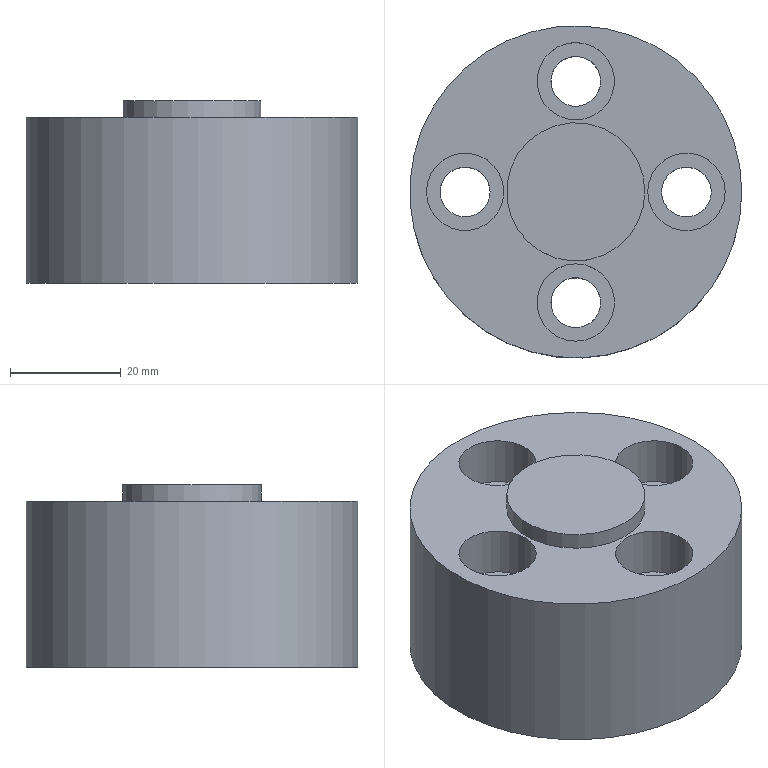Part | NX | 1 solid | 17 faces | box 60 x 60 x 33 mm | volume 75410 mm3 | cylinder 10 | plane 7 | commonest cylinder face diameters 9 x4 14 x4 25 x1 60 x1
STEP:
#1=CARTESIAN_POINT('',(0.,-24.5,-30.));
#2=VERTEX_POINT('',#1);
#3=CARTESIAN_POINT('',(0.,-20.,-30.));
#4=DIRECTION('',(0.,0.,1.));
#5=DIRECTION('',(0.,-1.,0.));
#6=AXIS2_PLACEMENT_3D('',#3,#4,#5);
#7=CIRCLE('',#6,4.5);
#8=EDGE_CURVE('',#2,#2,#7,.T.);
#9=ORIENTED_EDGE('',*,*,#8,.F.);
#10=EDGE_LOOP('',(#9));
#11=FACE_BOUND('',#10,.T.);
#12=CARTESIAN_POINT('',(4.5,-20.,-9.));
#13=VERTEX_POINT('',#12);
#14=CARTESIAN_POINT('',(0.,-20.,-9.));
#15=DIRECTION('',(0.,0.,1.));
#16=DIRECTION('',(1.,0.,0.));
#17=AXIS2_PLACEMENT_3D('',#14,#15,#16);
#18=CIRCLE('',#17,4.5);
#19=EDGE_CURVE('',#13,#13,#18,.F.);
#20=ORIENTED_EDGE('',*,*,#19,.F.);
#21=EDGE_LOOP('',(#20));
#22=FACE_BOUND('',#21,.T.);
#23=CARTESIAN_POINT('',(0.,-20.,-30.));
#24=DIRECTION('',(0.,0.,1.));
#25=DIRECTION('',(1.,0.,0.));
#26=AXIS2_PLACEMENT_3D('',#23,#24,#25);
#27=CYLINDRICAL_SURFACE('',#26,4.5);
#28=ADVANCED_FACE('',(#11,#22),#27,.F.);
#29=CARTESIAN_POINT('',(0.,24.5,-30.));
#30=VERTEX_POINT('',#29);
#31=CARTESIAN_POINT('',(0.,20.,-30.));
#32=DIRECTION('',(0.,0.,1.));
#33=DIRECTION('',(0.,1.,0.));
#34=AXIS2_PLACEMENT_3D('',#31,#32,#33);
#35=CIRCLE('',#34,4.5);
#36=EDGE_CURVE('',#30,#30,#35,.T.);
#37=ORIENTED_EDGE('',*,*,#36,.F.);
#38=EDGE_LOOP('',(#37));
#39=FACE_BOUND('',#38,.T.);
#40=CARTESIAN_POINT('',(4.5,20.,-9.));
#41=VERTEX_POINT('',#40);
#42=CARTESIAN_POINT('',(0.,20.,-9.));
#43=DIRECTION('',(0.,0.,1.));
#44=DIRECTION('',(1.,0.,0.));
#45=AXIS2_PLACEMENT_3D('',#42,#43,#44);
#46=CIRCLE('',#45,4.5);
#47=EDGE_CURVE('',#41,#41,#46,.F.);
#48=ORIENTED_EDGE('',*,*,#47,.F.);
#49=EDGE_LOOP('',(#48));
#50=FACE_BOUND('',#49,.T.);
#51=CARTESIAN_POINT('',(0.,20.,-30.));
#52=DIRECTION('',(0.,0.,1.));
#53=DIRECTION('',(1.,0.,0.));
#54=AXIS2_PLACEMENT_3D('',#51,#52,#53);
#55=CYLINDRICAL_SURFACE('',#54,4.5);
#56=ADVANCED_FACE('',(#39,#50),#55,.F.);
#57=CARTESIAN_POINT('',(24.5,0.,-30.));
#58=VERTEX_POINT('',#57);
#59=CARTESIAN_POINT('',(20.,0.,-30.));
#60=DIRECTION('',(0.,0.,1.));
#61=DIRECTION('',(1.,0.,0.));
#62=AXIS2_PLACEMENT_3D('',#59,#60,#61);
#63=CIRCLE('',#62,4.5);
#64=EDGE_CURVE('',#58,#58,#63,.T.);
#65=ORIENTED_EDGE('',*,*,#64,.F.);
#66=EDGE_LOOP('',(#65));
#67=FACE_BOUND('',#66,.T.);
#68=CARTESIAN_POINT('',(24.5,0.,-9.));
#69=VERTEX_POINT('',#68);
#70=CARTESIAN_POINT('',(20.,0.,-9.));
#71=DIRECTION('',(0.,0.,1.));
#72=DIRECTION('',(1.,0.,0.));
#73=AXIS2_PLACEMENT_3D('',#70,#71,#72);
#74=CIRCLE('',#73,4.5);
#75=EDGE_CURVE('',#69,#69,#74,.F.);
#76=ORIENTED_EDGE('',*,*,#75,.F.);
#77=EDGE_LOOP('',(#76));
#78=FACE_BOUND('',#77,.T.);
#79=CARTESIAN_POINT('',(20.,0.,-30.));
#80=DIRECTION('',(0.,0.,1.));
#81=DIRECTION('',(1.,0.,0.));
#82=AXIS2_PLACEMENT_3D('',#79,#80,#81);
#83=CYLINDRICAL_SURFACE('',#82,4.5);
#84=ADVANCED_FACE('',(#67,#78),#83,.F.);
#85=CARTESIAN_POINT('',(12.5,0.,0.));
#86=VERTEX_POINT('',#85);
#87=CARTESIAN_POINT('',(0.,0.,0.));
#88=DIRECTION('',(0.,0.,1.));
#89=DIRECTION('',(1.,0.,0.));
#90=AXIS2_PLACEMENT_3D('',#87,#88,#89);
#91=CIRCLE('',#90,12.5);
#92=EDGE_CURVE('',#86,#86,#91,.T.);
#93=ORIENTED_EDGE('',*,*,#92,.F.);
#94=EDGE_LOOP('',(#93));
#95=FACE_BOUND('',#94,.T.);
#96=CARTESIAN_POINT('',(0.,27.,0.));
#97=VERTEX_POINT('',#96);
#98=CARTESIAN_POINT('',(0.,20.,0.));
#99=DIRECTION('',(0.,0.,1.));
#100=DIRECTION('',(0.,1.,0.));
#101=AXIS2_PLACEMENT_3D('',#98,#99,#100);
#102=CIRCLE('',#101,7.);
#103=EDGE_CURVE('',#97,#97,#102,.T.);
#104=ORIENTED_EDGE('',*,*,#103,.F.);
#105=EDGE_LOOP('',(#104));
#106=FACE_BOUND('',#105,.T.);
#107=CARTESIAN_POINT('',(30.,0.,0.));
#108=VERTEX_POINT('',#107);
#109=CARTESIAN_POINT('',(0.,0.,0.));
#110=DIRECTION('',(0.,0.,1.));
#111=DIRECTION('',(1.,0.,0.));
#112=AXIS2_PLACEMENT_3D('',#109,#110,#111);
#113=CIRCLE('',#112,30.);
#114=EDGE_CURVE('',#108,#108,#113,.T.);
#115=ORIENTED_EDGE('',*,*,#114,.T.);
#116=EDGE_LOOP('',(#115));
#117=FACE_BOUND('',#116,.T.);
#118=CARTESIAN_POINT('',(-27.,0.,0.));
#119=VERTEX_POINT('',#118);
#120=CARTESIAN_POINT('',(-20.,0.,0.));
#121=DIRECTION('',(0.,0.,-1.));
#122=DIRECTION('',(-1.,0.,0.));
#123=AXIS2_PLACEMENT_3D('',#120,#121,#122);
#124=CIRCLE('',#123,7.);
#125=EDGE_CURVE('',#119,#119,#124,.T.);
#126=ORIENTED_EDGE('',*,*,#125,.T.);
#127=EDGE_LOOP('',(#126));
#128=FACE_BOUND('',#127,.T.);
#129=CARTESIAN_POINT('',(0.,-27.,0.));
#130=VERTEX_POINT('',#129);
#131=CARTESIAN_POINT('',(0.,-20.,0.));
#132=DIRECTION('',(0.,0.,1.));
#133=DIRECTION('',(0.,-1.,0.));
#134=AXIS2_PLACEMENT_3D('',#131,#132,#133);
#135=CIRCLE('',#134,7.);
#136=EDGE_CURVE('',#130,#130,#135,.T.);
#137=ORIENTED_EDGE('',*,*,#136,.F.);
#138=EDGE_LOOP('',(#137));
#139=FACE_BOUND('',#138,.T.);
#140=CARTESIAN_POINT('',(27.,0.,0.));
#141=VERTEX_POINT('',#140);
#142=CARTESIAN_POINT('',(20.,0.,0.));
#143=DIRECTION('',(0.,0.,1.));
#144=DIRECTION('',(1.,0.,0.));
#145=AXIS2_PLACEMENT_3D('',#142,#143,#144);
#146=CIRCLE('',#145,7.);
#147=EDGE_CURVE('',#141,#141,#146,.T.);
#148=ORIENTED_EDGE('',*,*,#147,.F.);
#149=EDGE_LOOP('',(#148));
#150=FACE_BOUND('',#149,.T.);
#151=CARTESIAN_POINT('',(10.,0.,0.));
#152=DIRECTION('',(0.,0.,1.));
#153=DIRECTION('',(1.,0.,0.));
#154=AXIS2_PLACEMENT_3D('',#151,#152,#153);
#155=PLANE('',#154);
#156=ADVANCED_FACE('',(#95,#106,#117,#128,#139,#150),#155,.T.);
#157=CARTESIAN_POINT('',(30.,0.,-30.));
#158=VERTEX_POINT('',#157);
#159=CARTESIAN_POINT('',(0.,0.,-30.));
#160=DIRECTION('',(0.,0.,1.));
#161=DIRECTION('',(1.,0.,0.));
#162=AXIS2_PLACEMENT_3D('',#159,#160,#161);
#163=CIRCLE('',#162,30.);
#164=EDGE_CURVE('',#158,#158,#163,.T.);
#165=ORIENTED_EDGE('',*,*,#164,.T.);
#166=EDGE_LOOP('',(#165));
#167=FACE_BOUND('',#166,.T.);
#168=ORIENTED_EDGE('',*,*,#114,.F.);
#169=EDGE_LOOP('',(#168));
#170=FACE_BOUND('',#169,.T.);
#171=CARTESIAN_POINT('',(0.,0.,-30.));
#172=DIRECTION('',(0.,0.,1.));
#173=DIRECTION('',(1.,0.,0.));
#174=AXIS2_PLACEMENT_3D('',#171,#172,#173);
#175=CYLINDRICAL_SURFACE('',#174,30.);
#176=ADVANCED_FACE('',(#167,#170),#175,.T.);
#177=CARTESIAN_POINT('',(-24.5,0.,-9.));
#178=VERTEX_POINT('',#177);
#179=CARTESIAN_POINT('',(-20.,0.,-9.));
#180=DIRECTION('',(0.,0.,-1.));
#181=DIRECTION('',(-1.,0.,0.));
#182=AXIS2_PLACEMENT_3D('',#179,#180,#181);
#183=CIRCLE('',#182,4.5);
#184=EDGE_CURVE('',#178,#178,#183,.F.);
#185=ORIENTED_EDGE('',*,*,#184,.T.);
#186=EDGE_LOOP('',(#185));
#187=FACE_BOUND('',#186,.T.);
#188=CARTESIAN_POINT('',(-24.5,0.,-30.));
#189=VERTEX_POINT('',#188);
#190=CARTESIAN_POINT('',(-20.,0.,-30.));
#191=DIRECTION('',(0.,0.,1.));
#192=DIRECTION('',(-1.,0.,0.));
#193=AXIS2_PLACEMENT_3D('',#190,#191,#192);
#194=CIRCLE('',#193,4.5);
#195=EDGE_CURVE('',#189,#189,#194,.T.);
#196=ORIENTED_EDGE('',*,*,#195,.F.);
#197=EDGE_LOOP('',(#196));
#198=FACE_BOUND('',#197,.T.);
#199=CARTESIAN_POINT('',(-20.,0.,-30.));
#200=DIRECTION('',(0.,0.,1.));
#201=DIRECTION('',(1.,0.,0.));
#202=AXIS2_PLACEMENT_3D('',#199,#200,#201);
#203=CYLINDRICAL_SURFACE('',#202,4.5);
#204=ADVANCED_FACE('',(#187,#198),#203,.F.);
#205=ORIENTED_EDGE('',*,*,#164,.F.);
#206=EDGE_LOOP('',(#205));
#207=FACE_BOUND('',#206,.T.);
#208=ORIENTED_EDGE('',*,*,#64,.T.);
#209=EDGE_LOOP('',(#208));
#210=FACE_BOUND('',#209,.T.);
#211=ORIENTED_EDGE('',*,*,#36,.T.);
#212=EDGE_LOOP('',(#211));
#213=FACE_BOUND('',#212,.T.);
#214=ORIENTED_EDGE('',*,*,#8,.T.);
#215=EDGE_LOOP('',(#214));
#216=FACE_BOUND('',#215,.T.);
#217=ORIENTED_EDGE('',*,*,#195,.T.);
#218=EDGE_LOOP('',(#217));
#219=FACE_BOUND('',#218,.T.);
#220=CARTESIAN_POINT('',(10.,0.,-30.));
#221=DIRECTION('',(0.,0.,1.));
#222=DIRECTION('',(1.,0.,0.));
#223=AXIS2_PLACEMENT_3D('',#220,#221,#222);
#224=PLANE('',#223);
#225=ADVANCED_FACE('',(#207,#210,#213,#216,#219),#224,.F.);
#226=CARTESIAN_POINT('',(-27.,0.,-9.));
#227=VERTEX_POINT('',#226);
#228=CARTESIAN_POINT('',(-20.,0.,-9.));
#229=DIRECTION('',(0.,0.,-1.));
#230=DIRECTION('',(-1.,0.,0.));
#231=AXIS2_PLACEMENT_3D('',#228,#229,#230);
#232=CIRCLE('',#231,7.);
#233=EDGE_CURVE('',#227,#227,#232,.F.);
#234=ORIENTED_EDGE('',*,*,#233,.T.);
#235=EDGE_LOOP('',(#234));
#236=FACE_BOUND('',#235,.T.);
#237=ORIENTED_EDGE('',*,*,#184,.F.);
#238=EDGE_LOOP('',(#237));
#239=FACE_BOUND('',#238,.T.);
#240=CARTESIAN_POINT('',(-20.,0.,-9.));
#241=DIRECTION('',(0.,0.,-1.));
#242=DIRECTION('',(-1.,0.,0.));
#243=AXIS2_PLACEMENT_3D('',#240,#241,#242);
#244=PLANE('',#243);
#245=ADVANCED_FACE('',(#236,#239),#244,.F.);
#246=ORIENTED_EDGE('',*,*,#233,.F.);
#247=EDGE_LOOP('',(#246));
#248=FACE_BOUND('',#247,.T.);
#249=ORIENTED_EDGE('',*,*,#125,.F.);
#250=EDGE_LOOP('',(#249));
#251=FACE_BOUND('',#250,.T.);
#252=CARTESIAN_POINT('',(-20.,0.,-9.));
#253=DIRECTION('',(0.,0.,1.));
#254=DIRECTION('',(1.,0.,0.));
#255=AXIS2_PLACEMENT_3D('',#252,#253,#254);
#256=CYLINDRICAL_SURFACE('',#255,7.);
#257=ADVANCED_FACE('',(#248,#251),#256,.F.);
#258=CARTESIAN_POINT('',(0.,-27.,-9.));
#259=VERTEX_POINT('',#258);
#260=CARTESIAN_POINT('',(0.,-20.,-9.));
#261=DIRECTION('',(0.,0.,1.));
#262=DIRECTION('',(0.,-1.,0.));
#263=AXIS2_PLACEMENT_3D('',#260,#261,#262);
#264=CIRCLE('',#263,7.);
#265=EDGE_CURVE('',#259,#259,#264,.F.);
#266=ORIENTED_EDGE('',*,*,#265,.F.);
#267=EDGE_LOOP('',(#266));
#268=FACE_BOUND('',#267,.T.);
#269=ORIENTED_EDGE('',*,*,#19,.T.);
#270=EDGE_LOOP('',(#269));
#271=FACE_BOUND('',#270,.T.);
#272=CARTESIAN_POINT('',(0.,-20.,-9.));
#273=DIRECTION('',(0.,0.,1.));
#274=DIRECTION('',(1.,0.,0.));
#275=AXIS2_PLACEMENT_3D('',#272,#273,#274);
#276=PLANE('',#275);
#277=ADVANCED_FACE('',(#268,#271),#276,.T.);
#278=ORIENTED_EDGE('',*,*,#265,.T.);
#279=EDGE_LOOP('',(#278));
#280=FACE_BOUND('',#279,.T.);
#281=ORIENTED_EDGE('',*,*,#136,.T.);
#282=EDGE_LOOP('',(#281));
#283=FACE_BOUND('',#282,.T.);
#284=CARTESIAN_POINT('',(0.,-20.,-9.));
#285=DIRECTION('',(0.,0.,1.));
#286=DIRECTION('',(1.,0.,0.));
#287=AXIS2_PLACEMENT_3D('',#284,#285,#286);
#288=CYLINDRICAL_SURFACE('',#287,7.);
#289=ADVANCED_FACE('',(#280,#283),#288,.F.);
#290=CARTESIAN_POINT('',(0.,27.,-9.));
#291=VERTEX_POINT('',#290);
#292=CARTESIAN_POINT('',(0.,20.,-9.));
#293=DIRECTION('',(0.,0.,1.));
#294=DIRECTION('',(0.,1.,0.));
#295=AXIS2_PLACEMENT_3D('',#292,#293,#294);
#296=CIRCLE('',#295,7.);
#297=EDGE_CURVE('',#291,#291,#296,.F.);
#298=ORIENTED_EDGE('',*,*,#297,.F.);
#299=EDGE_LOOP('',(#298));
#300=FACE_BOUND('',#299,.T.);
#301=ORIENTED_EDGE('',*,*,#47,.T.);
#302=EDGE_LOOP('',(#301));
#303=FACE_BOUND('',#302,.T.);
#304=CARTESIAN_POINT('',(0.,20.,-9.));
#305=DIRECTION('',(0.,0.,1.));
#306=DIRECTION('',(1.,0.,0.));
#307=AXIS2_PLACEMENT_3D('',#304,#305,#306);
#308=PLANE('',#307);
#309=ADVANCED_FACE('',(#300,#303),#308,.T.);
#310=ORIENTED_EDGE('',*,*,#297,.T.);
#311=EDGE_LOOP('',(#310));
#312=FACE_BOUND('',#311,.T.);
#313=ORIENTED_EDGE('',*,*,#103,.T.);
#314=EDGE_LOOP('',(#313));
#315=FACE_BOUND('',#314,.T.);
#316=CARTESIAN_POINT('',(0.,20.,-9.));
#317=DIRECTION('',(0.,0.,1.));
#318=DIRECTION('',(1.,0.,0.));
#319=AXIS2_PLACEMENT_3D('',#316,#317,#318);
#320=CYLINDRICAL_SURFACE('',#319,7.);
#321=ADVANCED_FACE('',(#312,#315),#320,.F.);
#322=CARTESIAN_POINT('',(27.,0.,-9.));
#323=VERTEX_POINT('',#322);
#324=CARTESIAN_POINT('',(20.,0.,-9.));
#325=DIRECTION('',(0.,0.,1.));
#326=DIRECTION('',(1.,0.,0.));
#327=AXIS2_PLACEMENT_3D('',#324,#325,#326);
#328=CIRCLE('',#327,7.);
#329=EDGE_CURVE('',#323,#323,#328,.F.);
#330=ORIENTED_EDGE('',*,*,#329,.F.);
#331=EDGE_LOOP('',(#330));
#332=FACE_BOUND('',#331,.T.);
#333=ORIENTED_EDGE('',*,*,#75,.T.);
#334=EDGE_LOOP('',(#333));
#335=FACE_BOUND('',#334,.T.);
#336=CARTESIAN_POINT('',(20.,0.,-9.));
#337=DIRECTION('',(0.,0.,1.));
#338=DIRECTION('',(1.,0.,0.));
#339=AXIS2_PLACEMENT_3D('',#336,#337,#338);
#340=PLANE('',#339);
#341=ADVANCED_FACE('',(#332,#335),#340,.T.);
#342=ORIENTED_EDGE('',*,*,#329,.T.);
#343=EDGE_LOOP('',(#342));
#344=FACE_BOUND('',#343,.T.);
#345=ORIENTED_EDGE('',*,*,#147,.T.);
#346=EDGE_LOOP('',(#345));
#347=FACE_BOUND('',#346,.T.);
#348=CARTESIAN_POINT('',(20.,0.,-9.));
#349=DIRECTION('',(0.,0.,1.));
#350=DIRECTION('',(1.,0.,0.));
#351=AXIS2_PLACEMENT_3D('',#348,#349,#350);
#352=CYLINDRICAL_SURFACE('',#351,7.);
#353=ADVANCED_FACE('',(#344,#347),#352,.F.);
#354=CARTESIAN_POINT('',(12.5,0.,3.));
#355=VERTEX_POINT('',#354);
#356=CARTESIAN_POINT('',(0.,0.,3.));
#357=DIRECTION('',(0.,0.,1.));
#358=DIRECTION('',(1.,0.,0.));
#359=AXIS2_PLACEMENT_3D('',#356,#357,#358);
#360=CIRCLE('',#359,12.5);
#361=EDGE_CURVE('',#355,#355,#360,.T.);
#362=ORIENTED_EDGE('',*,*,#361,.F.);
#363=EDGE_LOOP('',(#362));
#364=FACE_BOUND('',#363,.T.);
#365=ORIENTED_EDGE('',*,*,#92,.T.);
#366=EDGE_LOOP('',(#365));
#367=FACE_BOUND('',#366,.T.);
#368=CARTESIAN_POINT('',(0.,0.,3.));
#369=DIRECTION('',(0.,0.,-1.));
#370=DIRECTION('',(-1.,0.,0.));
#371=AXIS2_PLACEMENT_3D('',#368,#369,#370);
#372=CYLINDRICAL_SURFACE('',#371,12.5);
#373=ADVANCED_FACE('',(#364,#367),#372,.T.);
#374=ORIENTED_EDGE('',*,*,#361,.T.);
#375=EDGE_LOOP('',(#374));
#376=FACE_BOUND('',#375,.T.);
#377=CARTESIAN_POINT('',(0.,0.,3.));
#378=DIRECTION('',(0.,0.,1.));
#379=DIRECTION('',(1.,0.,0.));
#380=AXIS2_PLACEMENT_3D('',#377,#378,#379);
#381=PLANE('',#380);
#382=ADVANCED_FACE('',(#376),#381,.T.);
#383=CLOSED_SHELL('',(#28,#56,#84,#156,#176,#204,#225,#245,#257,#277,#289,#309,#321,#341,#353,#373,#382));
#384=MANIFOLD_SOLID_BREP('',#383);
#385=(LENGTH_UNIT()NAMED_UNIT(*)SI_UNIT(.MILLI.,.METRE.));
#386=UNCERTAINTY_MEASURE_WITH_UNIT(LENGTH_MEASURE(0.00001),#385,'','');
#387=(NAMED_UNIT(*)PLANE_ANGLE_UNIT()SI_UNIT($,.RADIAN.));
#388=(NAMED_UNIT(*)SI_UNIT($,.STERADIAN.)SOLID_ANGLE_UNIT());
#389=(GEOMETRIC_REPRESENTATION_CONTEXT(3)GLOBAL_UNCERTAINTY_ASSIGNED_CONTEXT((#386))GLOBAL_UNIT_ASSIGNED_CONTEXT((#385,#387,#388))REPRESENTATION_CONTEXT('',''));
#390=ADVANCED_BREP_SHAPE_REPRESENTATION('',(#384),#389);